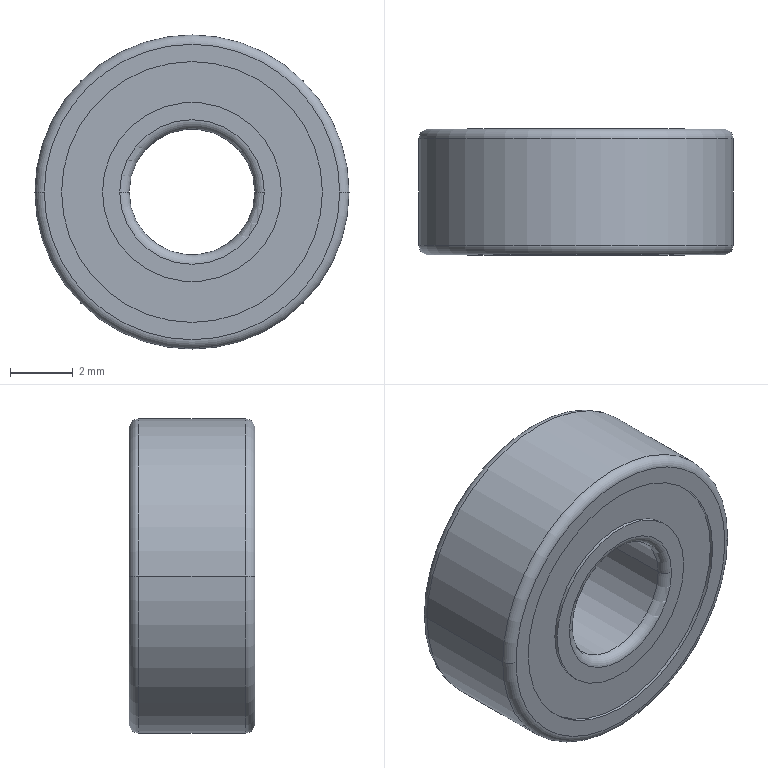Part | NX | 1 solid | 26 faces | box 10 x 4 x 10 mm | volume 256.477 mm3 | cylinder 12 | torus 8 | plane 6 | commonest cylinder face diameters 5.7 x4 8.3 x4 4 x2 10 x2
STEP:
#1=CARTESIAN_POINT('',(2.,1.7,0.));
#2=VERTEX_POINT('',#1);
#3=CARTESIAN_POINT('',(-2.,1.7,0.));
#4=VERTEX_POINT('',#3);
#5=CARTESIAN_POINT('',(0.,1.7,0.));
#6=DIRECTION('',(0.,-1.,0.));
#7=DIRECTION('',(-1.,0.,0.));
#8=AXIS2_PLACEMENT_3D('',#5,#6,#7);
#9=CIRCLE('',#8,2.);
#10=EDGE_CURVE('',#2,#4,#9,.T.);
#11=ORIENTED_EDGE('',*,*,#10,.T.);
#12=CARTESIAN_POINT('',(-2.3,2.,0.));
#13=VERTEX_POINT('',#12);
#14=CARTESIAN_POINT('',(-2.3,1.7,0.));
#15=DIRECTION('',(0.,0.,-1.));
#16=DIRECTION('',(-1.,0.,0.));
#17=AXIS2_PLACEMENT_3D('',#14,#15,#16);
#18=CIRCLE('',#17,0.3);
#19=EDGE_CURVE('',#4,#13,#18,.F.);
#20=ORIENTED_EDGE('',*,*,#19,.T.);
#21=CARTESIAN_POINT('',(2.3,2.,0.));
#22=VERTEX_POINT('',#21);
#23=CARTESIAN_POINT('',(0.,2.,0.));
#24=DIRECTION('',(0.,1.,0.));
#25=DIRECTION('',(1.,0.,0.));
#26=AXIS2_PLACEMENT_3D('',#23,#24,#25);
#27=CIRCLE('',#26,2.3);
#28=EDGE_CURVE('',#13,#22,#27,.T.);
#29=ORIENTED_EDGE('',*,*,#28,.T.);
#30=CARTESIAN_POINT('',(2.3,1.7,0.));
#31=DIRECTION('',(0.,0.,1.));
#32=DIRECTION('',(1.,0.,0.));
#33=AXIS2_PLACEMENT_3D('',#30,#31,#32);
#34=CIRCLE('',#33,0.3);
#35=EDGE_CURVE('',#2,#22,#34,.F.);
#36=ORIENTED_EDGE('',*,*,#35,.F.);
#37=EDGE_LOOP('',(#11,#20,#29,#36));
#38=FACE_BOUND('',#37,.T.);
#39=CARTESIAN_POINT('',(0.,1.7,0.));
#40=DIRECTION('',(0.,-1.,0.));
#41=DIRECTION('',(-1.,0.,0.));
#42=AXIS2_PLACEMENT_3D('',#39,#40,#41);
#43=TOROIDAL_SURFACE('',#42,2.3,0.3);
#44=ADVANCED_FACE('',(#38),#43,.T.);
#45=CARTESIAN_POINT('',(-2.85,2.,0.));
#46=VERTEX_POINT('',#45);
#47=CARTESIAN_POINT('',(2.85,2.,0.));
#48=VERTEX_POINT('',#47);
#49=CARTESIAN_POINT('',(0.,2.,0.));
#50=DIRECTION('',(0.,-1.,0.));
#51=DIRECTION('',(1.,0.,0.));
#52=AXIS2_PLACEMENT_3D('',#49,#50,#51);
#53=CIRCLE('',#52,2.85);
#54=EDGE_CURVE('',#46,#48,#53,.T.);
#55=ORIENTED_EDGE('',*,*,#54,.T.);
#56=CARTESIAN_POINT('',(2.85,1.9,0.));
#57=VERTEX_POINT('',#56);
#58=CARTESIAN_POINT('',(2.85,2.2,0.));
#59=DIRECTION('',(0.,-1.,0.));
#60=VECTOR('',#59,1000.);
#61=LINE('',#58,#60);
#62=EDGE_CURVE('',#48,#57,#61,.T.);
#63=ORIENTED_EDGE('',*,*,#62,.T.);
#64=CARTESIAN_POINT('',(-2.85,1.9,0.));
#65=VERTEX_POINT('',#64);
#66=CARTESIAN_POINT('',(0.,1.9,0.));
#67=DIRECTION('',(0.,1.,0.));
#68=DIRECTION('',(1.,0.,0.));
#69=AXIS2_PLACEMENT_3D('',#66,#67,#68);
#70=CIRCLE('',#69,2.85);
#71=EDGE_CURVE('',#57,#65,#70,.T.);
#72=ORIENTED_EDGE('',*,*,#71,.T.);
#73=CARTESIAN_POINT('',(-2.85,2.2,0.));
#74=DIRECTION('',(0.,-1.,0.));
#75=VECTOR('',#74,1000.);
#76=LINE('',#73,#75);
#77=EDGE_CURVE('',#46,#65,#76,.T.);
#78=ORIENTED_EDGE('',*,*,#77,.F.);
#79=EDGE_LOOP('',(#55,#63,#72,#78));
#80=FACE_BOUND('',#79,.T.);
#81=CARTESIAN_POINT('',(0.,2.2,0.));
#82=DIRECTION('',(0.,-1.,0.));
#83=DIRECTION('',(-1.,0.,0.));
#84=AXIS2_PLACEMENT_3D('',#81,#82,#83);
#85=CYLINDRICAL_SURFACE('',#84,2.85);
#86=ADVANCED_FACE('',(#80),#85,.T.);
#87=ORIENTED_EDGE('',*,*,#10,.F.);
#88=CARTESIAN_POINT('',(2.,-1.7,0.));
#89=VERTEX_POINT('',#88);
#90=CARTESIAN_POINT('',(2.,2.2,0.));
#91=DIRECTION('',(0.,-1.,0.));
#92=VECTOR('',#91,1000.);
#93=LINE('',#90,#92);
#94=EDGE_CURVE('',#89,#2,#93,.F.);
#95=ORIENTED_EDGE('',*,*,#94,.F.);
#96=CARTESIAN_POINT('',(-2.,-1.7,0.));
#97=VERTEX_POINT('',#96);
#98=CARTESIAN_POINT('',(0.,-1.7,0.));
#99=DIRECTION('',(0.,-1.,0.));
#100=DIRECTION('',(-1.,0.,0.));
#101=AXIS2_PLACEMENT_3D('',#98,#99,#100);
#102=CIRCLE('',#101,2.);
#103=EDGE_CURVE('',#89,#97,#102,.T.);
#104=ORIENTED_EDGE('',*,*,#103,.T.);
#105=CARTESIAN_POINT('',(-2.,2.2,0.));
#106=DIRECTION('',(0.,-1.,0.));
#107=VECTOR('',#106,1000.);
#108=LINE('',#105,#107);
#109=EDGE_CURVE('',#97,#4,#108,.F.);
#110=ORIENTED_EDGE('',*,*,#109,.T.);
#111=EDGE_LOOP('',(#87,#95,#104,#110));
#112=FACE_BOUND('',#111,.T.);
#113=CARTESIAN_POINT('',(0.,2.2,0.));
#114=DIRECTION('',(0.,-1.,0.));
#115=DIRECTION('',(-1.,0.,0.));
#116=AXIS2_PLACEMENT_3D('',#113,#114,#115);
#117=CYLINDRICAL_SURFACE('',#116,2.);
#118=ADVANCED_FACE('',(#112),#117,.F.);
#119=CARTESIAN_POINT('',(-4.7,2.,0.));
#120=VERTEX_POINT('',#119);
#121=CARTESIAN_POINT('',(4.7,2.,0.));
#122=VERTEX_POINT('',#121);
#123=CARTESIAN_POINT('',(0.,2.,0.));
#124=DIRECTION('',(0.,-1.,0.));
#125=DIRECTION('',(1.,0.,0.));
#126=AXIS2_PLACEMENT_3D('',#123,#124,#125);
#127=CIRCLE('',#126,4.7);
#128=EDGE_CURVE('',#120,#122,#127,.T.);
#129=ORIENTED_EDGE('',*,*,#128,.T.);
#130=CARTESIAN_POINT('',(5.,1.7,0.));
#131=VERTEX_POINT('',#130);
#132=CARTESIAN_POINT('',(4.7,1.7,0.));
#133=DIRECTION('',(0.,0.,1.));
#134=DIRECTION('',(1.,0.,0.));
#135=AXIS2_PLACEMENT_3D('',#132,#133,#134);
#136=CIRCLE('',#135,0.3);
#137=EDGE_CURVE('',#131,#122,#136,.T.);
#138=ORIENTED_EDGE('',*,*,#137,.F.);
#139=CARTESIAN_POINT('',(-5.,1.7,0.));
#140=VERTEX_POINT('',#139);
#141=CARTESIAN_POINT('',(0.,1.7,0.));
#142=DIRECTION('',(0.,-1.,0.));
#143=DIRECTION('',(-1.,0.,0.));
#144=AXIS2_PLACEMENT_3D('',#141,#142,#143);
#145=CIRCLE('',#144,5.);
#146=EDGE_CURVE('',#140,#131,#145,.T.);
#147=ORIENTED_EDGE('',*,*,#146,.F.);
#148=CARTESIAN_POINT('',(-4.7,1.7,0.));
#149=DIRECTION('',(0.,0.,-1.));
#150=DIRECTION('',(-1.,0.,0.));
#151=AXIS2_PLACEMENT_3D('',#148,#149,#150);
#152=CIRCLE('',#151,0.3);
#153=EDGE_CURVE('',#140,#120,#152,.T.);
#154=ORIENTED_EDGE('',*,*,#153,.T.);
#155=EDGE_LOOP('',(#129,#138,#147,#154));
#156=FACE_BOUND('',#155,.T.);
#157=CARTESIAN_POINT('',(0.,1.7,0.));
#158=DIRECTION('',(0.,-1.,0.));
#159=DIRECTION('',(-1.,0.,0.));
#160=AXIS2_PLACEMENT_3D('',#157,#158,#159);
#161=TOROIDAL_SURFACE('',#160,4.7,0.3);
#162=ADVANCED_FACE('',(#156),#161,.T.);
#163=CARTESIAN_POINT('',(-2.3,-2.,0.));
#164=VERTEX_POINT('',#163);
#165=CARTESIAN_POINT('',(2.3,-2.,0.));
#166=VERTEX_POINT('',#165);
#167=CARTESIAN_POINT('',(0.,-2.,0.));
#168=DIRECTION('',(0.,-1.,0.));
#169=DIRECTION('',(1.,0.,0.));
#170=AXIS2_PLACEMENT_3D('',#167,#168,#169);
#171=CIRCLE('',#170,2.3);
#172=EDGE_CURVE('',#164,#166,#171,.T.);
#173=ORIENTED_EDGE('',*,*,#172,.T.);
#174=CARTESIAN_POINT('',(2.3,-1.7,0.));
#175=DIRECTION('',(0.,0.,1.));
#176=DIRECTION('',(1.,0.,0.));
#177=AXIS2_PLACEMENT_3D('',#174,#175,#176);
#178=CIRCLE('',#177,0.3);
#179=EDGE_CURVE('',#89,#166,#178,.T.);
#180=ORIENTED_EDGE('',*,*,#179,.F.);
#181=CARTESIAN_POINT('',(0.,-1.7,0.));
#182=DIRECTION('',(0.,-1.,0.));
#183=DIRECTION('',(-1.,0.,0.));
#184=AXIS2_PLACEMENT_3D('',#181,#182,#183);
#185=CIRCLE('',#184,2.);
#186=EDGE_CURVE('',#97,#89,#185,.T.);
#187=ORIENTED_EDGE('',*,*,#186,.F.);
#188=CARTESIAN_POINT('',(-2.3,-1.7,0.));
#189=DIRECTION('',(0.,0.,-1.));
#190=DIRECTION('',(-1.,0.,0.));
#191=AXIS2_PLACEMENT_3D('',#188,#189,#190);
#192=CIRCLE('',#191,0.3);
#193=EDGE_CURVE('',#97,#164,#192,.T.);
#194=ORIENTED_EDGE('',*,*,#193,.T.);
#195=EDGE_LOOP('',(#173,#180,#187,#194));
#196=FACE_BOUND('',#195,.T.);
#197=CARTESIAN_POINT('',(0.,-1.7,0.));
#198=DIRECTION('',(0.,-1.,0.));
#199=DIRECTION('',(-1.,0.,0.));
#200=AXIS2_PLACEMENT_3D('',#197,#198,#199);
#201=TOROIDAL_SURFACE('',#200,2.3,0.3);
#202=ADVANCED_FACE('',(#196),#201,.T.);
#203=CARTESIAN_POINT('',(4.15,2.,0.));
#204=VERTEX_POINT('',#203);
#205=CARTESIAN_POINT('',(-4.15,2.,0.));
#206=VERTEX_POINT('',#205);
#207=CARTESIAN_POINT('',(0.,2.,0.));
#208=DIRECTION('',(0.,1.,0.));
#209=DIRECTION('',(1.,0.,0.));
#210=AXIS2_PLACEMENT_3D('',#207,#208,#209);
#211=CIRCLE('',#210,4.15);
#212=EDGE_CURVE('',#204,#206,#211,.T.);
#213=ORIENTED_EDGE('',*,*,#212,.T.);
#214=CARTESIAN_POINT('',(-4.15,1.9,0.));
#215=VERTEX_POINT('',#214);
#216=CARTESIAN_POINT('',(-4.15,2.2,0.));
#217=DIRECTION('',(0.,-1.,0.));
#218=VECTOR('',#217,1000.);
#219=LINE('',#216,#218);
#220=EDGE_CURVE('',#215,#206,#219,.F.);
#221=ORIENTED_EDGE('',*,*,#220,.F.);
#222=CARTESIAN_POINT('',(4.15,1.9,0.));
#223=VERTEX_POINT('',#222);
#224=CARTESIAN_POINT('',(0.,1.9,0.));
#225=DIRECTION('',(0.,-1.,0.));
#226=DIRECTION('',(1.,0.,0.));
#227=AXIS2_PLACEMENT_3D('',#224,#225,#226);
#228=CIRCLE('',#227,4.15);
#229=EDGE_CURVE('',#215,#223,#228,.T.);
#230=ORIENTED_EDGE('',*,*,#229,.T.);
#231=CARTESIAN_POINT('',(4.15,2.2,0.));
#232=DIRECTION('',(0.,-1.,0.));
#233=VECTOR('',#232,1000.);
#234=LINE('',#231,#233);
#235=EDGE_CURVE('',#223,#204,#234,.F.);
#236=ORIENTED_EDGE('',*,*,#235,.T.);
#237=EDGE_LOOP('',(#213,#221,#230,#236));
#238=FACE_BOUND('',#237,.T.);
#239=CARTESIAN_POINT('',(0.,2.2,0.));
#240=DIRECTION('',(0.,-1.,0.));
#241=DIRECTION('',(-1.,0.,0.));
#242=AXIS2_PLACEMENT_3D('',#239,#240,#241);
#243=CYLINDRICAL_SURFACE('',#242,4.15);
#244=ADVANCED_FACE('',(#238),#243,.F.);
#245=CARTESIAN_POINT('',(2.85,-2.,0.));
#246=VERTEX_POINT('',#245);
#247=CARTESIAN_POINT('',(-2.85,-2.,0.));
#248=VERTEX_POINT('',#247);
#249=CARTESIAN_POINT('',(0.,-2.,0.));
#250=DIRECTION('',(0.,1.,0.));
#251=DIRECTION('',(1.,0.,0.));
#252=AXIS2_PLACEMENT_3D('',#249,#250,#251);
#253=CIRCLE('',#252,2.85);
#254=EDGE_CURVE('',#246,#248,#253,.T.);
#255=ORIENTED_EDGE('',*,*,#254,.F.);
#256=CARTESIAN_POINT('',(0.,-2.,0.));
#257=DIRECTION('',(0.,1.,0.));
#258=DIRECTION('',(1.,0.,0.));
#259=AXIS2_PLACEMENT_3D('',#256,#257,#258);
#260=CIRCLE('',#259,2.85);
#261=EDGE_CURVE('',#248,#246,#260,.T.);
#262=ORIENTED_EDGE('',*,*,#261,.F.);
#263=EDGE_LOOP('',(#255,#262));
#264=FACE_BOUND('',#263,.T.);
#265=ORIENTED_EDGE('',*,*,#172,.F.);
#266=CARTESIAN_POINT('',(0.,-2.,0.));
#267=DIRECTION('',(0.,-1.,0.));
#268=DIRECTION('',(1.,0.,0.));
#269=AXIS2_PLACEMENT_3D('',#266,#267,#268);
#270=CIRCLE('',#269,2.3);
#271=EDGE_CURVE('',#166,#164,#270,.T.);
#272=ORIENTED_EDGE('',*,*,#271,.F.);
#273=EDGE_LOOP('',(#265,#272));
#274=FACE_BOUND('',#273,.T.);
#275=CARTESIAN_POINT('',(0.,-2.,0.));
#276=DIRECTION('',(0.,-1.,0.));
#277=DIRECTION('',(0.,0.,-1.));
#278=AXIS2_PLACEMENT_3D('',#275,#276,#277);
#279=PLANE('',#278);
#280=ADVANCED_FACE('',(#264,#274),#279,.T.);
#281=CARTESIAN_POINT('',(2.85,-1.9,0.));
#282=VERTEX_POINT('',#281);
#283=CARTESIAN_POINT('',(-2.85,-1.9,0.));
#284=VERTEX_POINT('',#283);
#285=CARTESIAN_POINT('',(0.,-1.9,0.));
#286=DIRECTION('',(0.,-1.,0.));
#287=DIRECTION('',(1.,0.,0.));
#288=AXIS2_PLACEMENT_3D('',#285,#286,#287);
#289=CIRCLE('',#288,2.85);
#290=EDGE_CURVE('',#282,#284,#289,.T.);
#291=ORIENTED_EDGE('',*,*,#290,.T.);
#292=CARTESIAN_POINT('',(-2.85,2.2,0.));
#293=DIRECTION('',(0.,-1.,0.));
#294=VECTOR('',#293,1000.);
#295=LINE('',#292,#294);
#296=EDGE_CURVE('',#248,#284,#295,.F.);
#297=ORIENTED_EDGE('',*,*,#296,.F.);
#298=ORIENTED_EDGE('',*,*,#261,.T.);
#299=CARTESIAN_POINT('',(2.85,2.2,0.));
#300=DIRECTION('',(0.,-1.,0.));
#301=VECTOR('',#300,1000.);
#302=LINE('',#299,#301);
#303=EDGE_CURVE('',#246,#282,#302,.F.);
#304=ORIENTED_EDGE('',*,*,#303,.T.);
#305=EDGE_LOOP('',(#291,#297,#298,#304));
#306=FACE_BOUND('',#305,.T.);
#307=CARTESIAN_POINT('',(0.,2.2,0.));
#308=DIRECTION('',(0.,-1.,0.));
#309=DIRECTION('',(-1.,0.,0.));
#310=AXIS2_PLACEMENT_3D('',#307,#308,#309);
#311=CYLINDRICAL_SURFACE('',#310,2.85);
#312=ADVANCED_FACE('',(#306),#311,.T.);
#313=ORIENTED_EDGE('',*,*,#229,.F.);
#314=CARTESIAN_POINT('',(0.,1.9,0.));
#315=DIRECTION('',(0.,-1.,0.));
#316=DIRECTION('',(1.,0.,0.));
#317=AXIS2_PLACEMENT_3D('',#314,#315,#316);
#318=CIRCLE('',#317,4.15);
#319=EDGE_CURVE('',#223,#215,#318,.T.);
#320=ORIENTED_EDGE('',*,*,#319,.F.);
#321=EDGE_LOOP('',(#313,#320));
#322=FACE_BOUND('',#321,.T.);
#323=CARTESIAN_POINT('',(0.,1.9,0.));
#324=DIRECTION('',(0.,1.,0.));
#325=DIRECTION('',(1.,0.,0.));
#326=AXIS2_PLACEMENT_3D('',#323,#324,#325);
#327=CIRCLE('',#326,2.85);
#328=EDGE_CURVE('',#65,#57,#327,.T.);
#329=ORIENTED_EDGE('',*,*,#328,.F.);
#330=ORIENTED_EDGE('',*,*,#71,.F.);
#331=EDGE_LOOP('',(#329,#330));
#332=FACE_BOUND('',#331,.T.);
#333=CARTESIAN_POINT('',(0.,1.9,0.));
#334=DIRECTION('',(0.,-1.,0.));
#335=DIRECTION('',(0.,0.,-1.));
#336=AXIS2_PLACEMENT_3D('',#333,#334,#335);
#337=PLANE('',#336);
#338=ADVANCED_FACE('',(#322,#332),#337,.F.);
#339=CARTESIAN_POINT('',(4.15,-1.9,0.));
#340=VERTEX_POINT('',#339);
#341=CARTESIAN_POINT('',(-4.15,-1.9,0.));
#342=VERTEX_POINT('',#341);
#343=CARTESIAN_POINT('',(0.,-1.9,0.));
#344=DIRECTION('',(0.,1.,0.));
#345=DIRECTION('',(1.,0.,0.));
#346=AXIS2_PLACEMENT_3D('',#343,#344,#345);
#347=CIRCLE('',#346,4.15);
#348=EDGE_CURVE('',#340,#342,#347,.T.);
#349=ORIENTED_EDGE('',*,*,#348,.F.);
#350=CARTESIAN_POINT('',(0.,-1.9,0.));
#351=DIRECTION('',(0.,1.,0.));
#352=DIRECTION('',(1.,0.,0.));
#353=AXIS2_PLACEMENT_3D('',#350,#351,#352);
#354=CIRCLE('',#353,4.15);
#355=EDGE_CURVE('',#342,#340,#354,.T.);
#356=ORIENTED_EDGE('',*,*,#355,.F.);
#357=EDGE_LOOP('',(#349,#356));
#358=FACE_BOUND('',#357,.T.);
#359=ORIENTED_EDGE('',*,*,#290,.F.);
#360=CARTESIAN_POINT('',(0.,-1.9,0.));
#361=DIRECTION('',(0.,-1.,0.));
#362=DIRECTION('',(1.,0.,0.));
#363=AXIS2_PLACEMENT_3D('',#360,#361,#362);
#364=CIRCLE('',#363,2.85);
#365=EDGE_CURVE('',#284,#282,#364,.T.);
#366=ORIENTED_EDGE('',*,*,#365,.F.);
#367=EDGE_LOOP('',(#359,#366));
#368=FACE_BOUND('',#367,.T.);
#369=CARTESIAN_POINT('',(0.,-1.9,0.));
#370=DIRECTION('',(0.,-1.,0.));
#371=DIRECTION('',(0.,0.,-1.));
#372=AXIS2_PLACEMENT_3D('',#369,#370,#371);
#373=PLANE('',#372);
#374=ADVANCED_FACE('',(#358,#368),#373,.T.);
#375=CARTESIAN_POINT('',(4.15,-2.,0.));
#376=VERTEX_POINT('',#375);
#377=CARTESIAN_POINT('',(-4.15,-2.,0.));
#378=VERTEX_POINT('',#377);
#379=CARTESIAN_POINT('',(0.,-2.,0.));
#380=DIRECTION('',(0.,-1.,0.));
#381=DIRECTION('',(1.,0.,0.));
#382=AXIS2_PLACEMENT_3D('',#379,#380,#381);
#383=CIRCLE('',#382,4.15);
#384=EDGE_CURVE('',#376,#378,#383,.T.);
#385=ORIENTED_EDGE('',*,*,#384,.T.);
#386=CARTESIAN_POINT('',(-4.15,2.2,0.));
#387=DIRECTION('',(0.,-1.,0.));
#388=VECTOR('',#387,1000.);
#389=LINE('',#386,#388);
#390=EDGE_CURVE('',#378,#342,#389,.F.);
#391=ORIENTED_EDGE('',*,*,#390,.T.);
#392=ORIENTED_EDGE('',*,*,#355,.T.);
#393=CARTESIAN_POINT('',(4.15,2.2,0.));
#394=DIRECTION('',(0.,-1.,0.));
#395=VECTOR('',#394,1000.);
#396=LINE('',#393,#395);
#397=EDGE_CURVE('',#376,#340,#396,.F.);
#398=ORIENTED_EDGE('',*,*,#397,.F.);
#399=EDGE_LOOP('',(#385,#391,#392,#398));
#400=FACE_BOUND('',#399,.T.);
#401=CARTESIAN_POINT('',(0.,2.2,0.));
#402=DIRECTION('',(0.,-1.,0.));
#403=DIRECTION('',(-1.,0.,0.));
#404=AXIS2_PLACEMENT_3D('',#401,#402,#403);
#405=CYLINDRICAL_SURFACE('',#404,4.15);
#406=ADVANCED_FACE('',(#400),#405,.F.);
#407=ORIENTED_EDGE('',*,*,#54,.F.);
#408=CARTESIAN_POINT('',(0.,2.,0.));
#409=DIRECTION('',(0.,-1.,0.));
#410=DIRECTION('',(1.,0.,0.));
#411=AXIS2_PLACEMENT_3D('',#408,#409,#410);
#412=CIRCLE('',#411,2.85);
#413=EDGE_CURVE('',#48,#46,#412,.T.);
#414=ORIENTED_EDGE('',*,*,#413,.F.);
#415=EDGE_LOOP('',(#407,#414));
#416=FACE_BOUND('',#415,.T.);
#417=ORIENTED_EDGE('',*,*,#28,.F.);
#418=CARTESIAN_POINT('',(0.,2.,0.));
#419=DIRECTION('',(0.,1.,0.));
#420=DIRECTION('',(1.,0.,0.));
#421=AXIS2_PLACEMENT_3D('',#418,#419,#420);
#422=CIRCLE('',#421,2.3);
#423=EDGE_CURVE('',#22,#13,#422,.T.);
#424=ORIENTED_EDGE('',*,*,#423,.F.);
#425=EDGE_LOOP('',(#417,#424));
#426=FACE_BOUND('',#425,.T.);
#427=CARTESIAN_POINT('',(0.,2.,0.));
#428=DIRECTION('',(0.,-1.,0.));
#429=DIRECTION('',(0.,0.,-1.));
#430=AXIS2_PLACEMENT_3D('',#427,#428,#429);
#431=PLANE('',#430);
#432=ADVANCED_FACE('',(#416,#426),#431,.F.);
#433=CARTESIAN_POINT('',(4.7,-2.,0.));
#434=VERTEX_POINT('',#433);
#435=CARTESIAN_POINT('',(-4.7,-2.,0.));
#436=VERTEX_POINT('',#435);
#437=CARTESIAN_POINT('',(0.,-2.,0.));
#438=DIRECTION('',(0.,1.,0.));
#439=DIRECTION('',(1.,0.,0.));
#440=AXIS2_PLACEMENT_3D('',#437,#438,#439);
#441=CIRCLE('',#440,4.7);
#442=EDGE_CURVE('',#434,#436,#441,.T.);
#443=ORIENTED_EDGE('',*,*,#442,.F.);
#444=CARTESIAN_POINT('',(0.,-2.,0.));
#445=DIRECTION('',(0.,1.,0.));
#446=DIRECTION('',(1.,0.,0.));
#447=AXIS2_PLACEMENT_3D('',#444,#445,#446);
#448=CIRCLE('',#447,4.7);
#449=EDGE_CURVE('',#436,#434,#448,.T.);
#450=ORIENTED_EDGE('',*,*,#449,.F.);
#451=EDGE_LOOP('',(#443,#450));
#452=FACE_BOUND('',#451,.T.);
#453=ORIENTED_EDGE('',*,*,#384,.F.);
#454=CARTESIAN_POINT('',(0.,-2.,0.));
#455=DIRECTION('',(0.,-1.,0.));
#456=DIRECTION('',(1.,0.,0.));
#457=AXIS2_PLACEMENT_3D('',#454,#455,#456);
#458=CIRCLE('',#457,4.15);
#459=EDGE_CURVE('',#378,#376,#458,.T.);
#460=ORIENTED_EDGE('',*,*,#459,.F.);
#461=EDGE_LOOP('',(#453,#460));
#462=FACE_BOUND('',#461,.T.);
#463=CARTESIAN_POINT('',(0.,-2.,0.));
#464=DIRECTION('',(0.,-1.,0.));
#465=DIRECTION('',(0.,0.,-1.));
#466=AXIS2_PLACEMENT_3D('',#463,#464,#465);
#467=PLANE('',#466);
#468=ADVANCED_FACE('',(#452,#462),#467,.T.);
#469=CARTESIAN_POINT('',(-5.,-1.7,0.));
#470=VERTEX_POINT('',#469);
#471=CARTESIAN_POINT('',(5.,-1.7,0.));
#472=VERTEX_POINT('',#471);
#473=CARTESIAN_POINT('',(0.,-1.7,0.));
#474=DIRECTION('',(0.,-1.,0.));
#475=DIRECTION('',(-1.,0.,0.));
#476=AXIS2_PLACEMENT_3D('',#473,#474,#475);
#477=CIRCLE('',#476,5.);
#478=EDGE_CURVE('',#470,#472,#477,.T.);
#479=ORIENTED_EDGE('',*,*,#478,.T.);
#480=CARTESIAN_POINT('',(4.7,-1.7,0.));
#481=DIRECTION('',(0.,0.,1.));
#482=DIRECTION('',(1.,0.,0.));
#483=AXIS2_PLACEMENT_3D('',#480,#481,#482);
#484=CIRCLE('',#483,0.3);
#485=EDGE_CURVE('',#472,#434,#484,.F.);
#486=ORIENTED_EDGE('',*,*,#485,.T.);
#487=ORIENTED_EDGE('',*,*,#442,.T.);
#488=CARTESIAN_POINT('',(-4.7,-1.7,0.));
#489=DIRECTION('',(0.,0.,-1.));
#490=DIRECTION('',(-1.,0.,0.));
#491=AXIS2_PLACEMENT_3D('',#488,#489,#490);
#492=CIRCLE('',#491,0.3);
#493=EDGE_CURVE('',#470,#436,#492,.F.);
#494=ORIENTED_EDGE('',*,*,#493,.F.);
#495=EDGE_LOOP('',(#479,#486,#487,#494));
#496=FACE_BOUND('',#495,.T.);
#497=CARTESIAN_POINT('',(0.,-1.7,0.));
#498=DIRECTION('',(0.,-1.,0.));
#499=DIRECTION('',(-1.,0.,0.));
#500=AXIS2_PLACEMENT_3D('',#497,#498,#499);
#501=TOROIDAL_SURFACE('',#500,4.7,0.3);
#502=ADVANCED_FACE('',(#496),#501,.T.);
#503=ORIENTED_EDGE('',*,*,#128,.F.);
#504=CARTESIAN_POINT('',(0.,2.,0.));
#505=DIRECTION('',(0.,-1.,0.));
#506=DIRECTION('',(1.,0.,0.));
#507=AXIS2_PLACEMENT_3D('',#504,#505,#506);
#508=CIRCLE('',#507,4.7);
#509=EDGE_CURVE('',#122,#120,#508,.T.);
#510=ORIENTED_EDGE('',*,*,#509,.F.);
#511=EDGE_LOOP('',(#503,#510));
#512=FACE_BOUND('',#511,.T.);
#513=ORIENTED_EDGE('',*,*,#212,.F.);
#514=CARTESIAN_POINT('',(0.,2.,0.));
#515=DIRECTION('',(0.,1.,0.));
#516=DIRECTION('',(1.,0.,0.));
#517=AXIS2_PLACEMENT_3D('',#514,#515,#516);
#518=CIRCLE('',#517,4.15);
#519=EDGE_CURVE('',#206,#204,#518,.T.);
#520=ORIENTED_EDGE('',*,*,#519,.F.);
#521=EDGE_LOOP('',(#513,#520));
#522=FACE_BOUND('',#521,.T.);
#523=CARTESIAN_POINT('',(0.,2.,0.));
#524=DIRECTION('',(0.,-1.,0.));
#525=DIRECTION('',(0.,0.,-1.));
#526=AXIS2_PLACEMENT_3D('',#523,#524,#525);
#527=PLANE('',#526);
#528=ADVANCED_FACE('',(#512,#522),#527,.F.);
#529=ORIENTED_EDGE('',*,*,#478,.F.);
#530=CARTESIAN_POINT('',(-5.,2.2,0.));
#531=DIRECTION('',(0.,-1.,0.));
#532=VECTOR('',#531,1000.);
#533=LINE('',#530,#532);
#534=EDGE_CURVE('',#470,#140,#533,.F.);
#535=ORIENTED_EDGE('',*,*,#534,.T.);
#536=ORIENTED_EDGE('',*,*,#146,.T.);
#537=CARTESIAN_POINT('',(5.,2.2,0.));
#538=DIRECTION('',(0.,-1.,0.));
#539=VECTOR('',#538,1000.);
#540=LINE('',#537,#539);
#541=EDGE_CURVE('',#472,#131,#540,.F.);
#542=ORIENTED_EDGE('',*,*,#541,.F.);
#543=EDGE_LOOP('',(#529,#535,#536,#542));
#544=FACE_BOUND('',#543,.T.);
#545=CARTESIAN_POINT('',(0.,2.2,0.));
#546=DIRECTION('',(0.,-1.,0.));
#547=DIRECTION('',(-1.,0.,0.));
#548=AXIS2_PLACEMENT_3D('',#545,#546,#547);
#549=CYLINDRICAL_SURFACE('',#548,5.);
#550=ADVANCED_FACE('',(#544),#549,.T.);
#551=ORIENTED_EDGE('',*,*,#109,.F.);
#552=ORIENTED_EDGE('',*,*,#186,.T.);
#553=ORIENTED_EDGE('',*,*,#94,.T.);
#554=CARTESIAN_POINT('',(0.,1.7,0.));
#555=DIRECTION('',(0.,-1.,0.));
#556=DIRECTION('',(-1.,0.,0.));
#557=AXIS2_PLACEMENT_3D('',#554,#555,#556);
#558=CIRCLE('',#557,2.);
#559=EDGE_CURVE('',#4,#2,#558,.T.);
#560=ORIENTED_EDGE('',*,*,#559,.F.);
#561=EDGE_LOOP('',(#551,#552,#553,#560));
#562=FACE_BOUND('',#561,.T.);
#563=CARTESIAN_POINT('',(0.,2.2,0.));
#564=DIRECTION('',(0.,-1.,0.));
#565=DIRECTION('',(-1.,0.,0.));
#566=AXIS2_PLACEMENT_3D('',#563,#564,#565);
#567=CYLINDRICAL_SURFACE('',#566,2.);
#568=ADVANCED_FACE('',(#562),#567,.F.);
#569=ORIENTED_EDGE('',*,*,#328,.T.);
#570=ORIENTED_EDGE('',*,*,#62,.F.);
#571=ORIENTED_EDGE('',*,*,#413,.T.);
#572=ORIENTED_EDGE('',*,*,#77,.T.);
#573=EDGE_LOOP('',(#569,#570,#571,#572));
#574=FACE_BOUND('',#573,.T.);
#575=CARTESIAN_POINT('',(0.,2.2,0.));
#576=DIRECTION('',(0.,-1.,0.));
#577=DIRECTION('',(-1.,0.,0.));
#578=AXIS2_PLACEMENT_3D('',#575,#576,#577);
#579=CYLINDRICAL_SURFACE('',#578,2.85);
#580=ADVANCED_FACE('',(#574),#579,.T.);
#581=ORIENTED_EDGE('',*,*,#348,.T.);
#582=ORIENTED_EDGE('',*,*,#390,.F.);
#583=ORIENTED_EDGE('',*,*,#459,.T.);
#584=ORIENTED_EDGE('',*,*,#397,.T.);
#585=EDGE_LOOP('',(#581,#582,#583,#584));
#586=FACE_BOUND('',#585,.T.);
#587=CARTESIAN_POINT('',(0.,2.2,0.));
#588=DIRECTION('',(0.,-1.,0.));
#589=DIRECTION('',(-1.,0.,0.));
#590=AXIS2_PLACEMENT_3D('',#587,#588,#589);
#591=CYLINDRICAL_SURFACE('',#590,4.15);
#592=ADVANCED_FACE('',(#586),#591,.F.);
#593=ORIENTED_EDGE('',*,*,#220,.T.);
#594=ORIENTED_EDGE('',*,*,#519,.T.);
#595=ORIENTED_EDGE('',*,*,#235,.F.);
#596=ORIENTED_EDGE('',*,*,#319,.T.);
#597=EDGE_LOOP('',(#593,#594,#595,#596));
#598=FACE_BOUND('',#597,.T.);
#599=CARTESIAN_POINT('',(0.,2.2,0.));
#600=DIRECTION('',(0.,-1.,0.));
#601=DIRECTION('',(-1.,0.,0.));
#602=AXIS2_PLACEMENT_3D('',#599,#600,#601);
#603=CYLINDRICAL_SURFACE('',#602,4.15);
#604=ADVANCED_FACE('',(#598),#603,.F.);
#605=ORIENTED_EDGE('',*,*,#254,.T.);
#606=ORIENTED_EDGE('',*,*,#296,.T.);
#607=ORIENTED_EDGE('',*,*,#365,.T.);
#608=ORIENTED_EDGE('',*,*,#303,.F.);
#609=EDGE_LOOP('',(#605,#606,#607,#608));
#610=FACE_BOUND('',#609,.T.);
#611=CARTESIAN_POINT('',(0.,2.2,0.));
#612=DIRECTION('',(0.,-1.,0.));
#613=DIRECTION('',(-1.,0.,0.));
#614=AXIS2_PLACEMENT_3D('',#611,#612,#613);
#615=CYLINDRICAL_SURFACE('',#614,2.85);
#616=ADVANCED_FACE('',(#610),#615,.T.);
#617=CARTESIAN_POINT('',(0.,1.7,0.));
#618=DIRECTION('',(0.,-1.,0.));
#619=DIRECTION('',(-1.,0.,0.));
#620=AXIS2_PLACEMENT_3D('',#617,#618,#619);
#621=CIRCLE('',#620,5.);
#622=EDGE_CURVE('',#131,#140,#621,.T.);
#623=ORIENTED_EDGE('',*,*,#622,.T.);
#624=ORIENTED_EDGE('',*,*,#534,.F.);
#625=CARTESIAN_POINT('',(0.,-1.7,0.));
#626=DIRECTION('',(0.,-1.,0.));
#627=DIRECTION('',(-1.,0.,0.));
#628=AXIS2_PLACEMENT_3D('',#625,#626,#627);
#629=CIRCLE('',#628,5.);
#630=EDGE_CURVE('',#472,#470,#629,.T.);
#631=ORIENTED_EDGE('',*,*,#630,.F.);
#632=ORIENTED_EDGE('',*,*,#541,.T.);
#633=EDGE_LOOP('',(#623,#624,#631,#632));
#634=FACE_BOUND('',#633,.T.);
#635=CARTESIAN_POINT('',(0.,2.2,0.));
#636=DIRECTION('',(0.,-1.,0.));
#637=DIRECTION('',(-1.,0.,0.));
#638=AXIS2_PLACEMENT_3D('',#635,#636,#637);
#639=CYLINDRICAL_SURFACE('',#638,5.);
#640=ADVANCED_FACE('',(#634),#639,.T.);
#641=ORIENTED_EDGE('',*,*,#493,.T.);
#642=ORIENTED_EDGE('',*,*,#449,.T.);
#643=ORIENTED_EDGE('',*,*,#485,.F.);
#644=ORIENTED_EDGE('',*,*,#630,.T.);
#645=EDGE_LOOP('',(#641,#642,#643,#644));
#646=FACE_BOUND('',#645,.T.);
#647=CARTESIAN_POINT('',(0.,-1.7,0.));
#648=DIRECTION('',(0.,-1.,0.));
#649=DIRECTION('',(-1.,0.,0.));
#650=AXIS2_PLACEMENT_3D('',#647,#648,#649);
#651=TOROIDAL_SURFACE('',#650,4.7,0.3);
#652=ADVANCED_FACE('',(#646),#651,.T.);
#653=ORIENTED_EDGE('',*,*,#19,.F.);
#654=ORIENTED_EDGE('',*,*,#559,.T.);
#655=ORIENTED_EDGE('',*,*,#35,.T.);
#656=ORIENTED_EDGE('',*,*,#423,.T.);
#657=EDGE_LOOP('',(#653,#654,#655,#656));
#658=FACE_BOUND('',#657,.T.);
#659=CARTESIAN_POINT('',(0.,1.7,0.));
#660=DIRECTION('',(0.,-1.,0.));
#661=DIRECTION('',(-1.,0.,0.));
#662=AXIS2_PLACEMENT_3D('',#659,#660,#661);
#663=TOROIDAL_SURFACE('',#662,2.3,0.3);
#664=ADVANCED_FACE('',(#658),#663,.T.);
#665=ORIENTED_EDGE('',*,*,#622,.F.);
#666=ORIENTED_EDGE('',*,*,#137,.T.);
#667=ORIENTED_EDGE('',*,*,#509,.T.);
#668=ORIENTED_EDGE('',*,*,#153,.F.);
#669=EDGE_LOOP('',(#665,#666,#667,#668));
#670=FACE_BOUND('',#669,.T.);
#671=CARTESIAN_POINT('',(0.,1.7,0.));
#672=DIRECTION('',(0.,-1.,0.));
#673=DIRECTION('',(-1.,0.,0.));
#674=AXIS2_PLACEMENT_3D('',#671,#672,#673);
#675=TOROIDAL_SURFACE('',#674,4.7,0.3);
#676=ADVANCED_FACE('',(#670),#675,.T.);
#677=ORIENTED_EDGE('',*,*,#103,.F.);
#678=ORIENTED_EDGE('',*,*,#179,.T.);
#679=ORIENTED_EDGE('',*,*,#271,.T.);
#680=ORIENTED_EDGE('',*,*,#193,.F.);
#681=EDGE_LOOP('',(#677,#678,#679,#680));
#682=FACE_BOUND('',#681,.T.);
#683=CARTESIAN_POINT('',(0.,-1.7,0.));
#684=DIRECTION('',(0.,-1.,0.));
#685=DIRECTION('',(-1.,0.,0.));
#686=AXIS2_PLACEMENT_3D('',#683,#684,#685);
#687=TOROIDAL_SURFACE('',#686,2.3,0.3);
#688=ADVANCED_FACE('',(#682),#687,.T.);
#689=CLOSED_SHELL('',(#44,#86,#118,#162,#202,#244,#280,#312,#338,#374,#406,#432,#468,#502,#528,#550,#568,#580,#592,#604,#616,#640,#652,#664,#676,#688));
#690=MANIFOLD_SOLID_BREP('',#689);
#691=(LENGTH_UNIT()NAMED_UNIT(*)SI_UNIT(.MILLI.,.METRE.));
#692=UNCERTAINTY_MEASURE_WITH_UNIT(LENGTH_MEASURE(0.00001),#691,'','');
#693=(NAMED_UNIT(*)PLANE_ANGLE_UNIT()SI_UNIT($,.RADIAN.));
#694=(NAMED_UNIT(*)SI_UNIT($,.STERADIAN.)SOLID_ANGLE_UNIT());
#695=(GEOMETRIC_REPRESENTATION_CONTEXT(3)GLOBAL_UNCERTAINTY_ASSIGNED_CONTEXT((#692))GLOBAL_UNIT_ASSIGNED_CONTEXT((#691,#693,#694))REPRESENTATION_CONTEXT('',''));
#696=ADVANCED_BREP_SHAPE_REPRESENTATION('',(#690),#695);